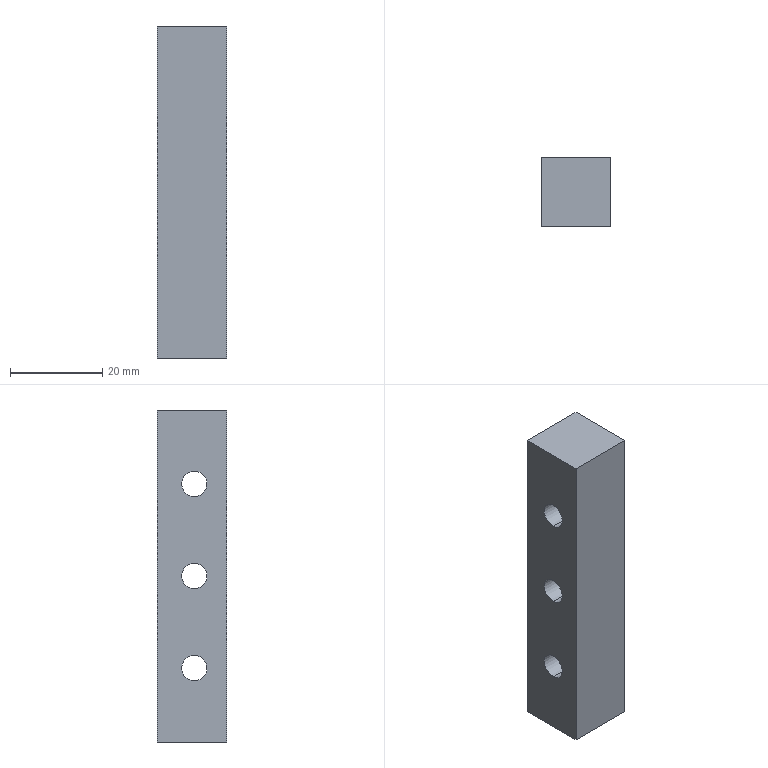Part | SolidWorks | features Extrusion 1, HoleWzd 1 | 1 solid | 21 faces | box 15 x 15 x 72 mm | volume 14194 mm3 | cylinder 12 | plane 9 | commonest cylinder face diameters 5.5 x6 10 x6
STEP:
#1=CARTESIAN_POINT('',(9.3,-0.5,25.));
#2=VERTEX_POINT('',#1);
#3=CARTESIAN_POINT('',(9.3,-0.5,15.));
#4=VERTEX_POINT('',#3);
#5=CARTESIAN_POINT('',(9.3,-0.5,20.));
#6=DIRECTION('',(1.,0.,0.));
#7=DIRECTION('',(0.,0.,-1.));
#8=AXIS2_PLACEMENT_3D('',#5,#6,#7);
#9=CIRCLE('',#8,5.);
#10=EDGE_CURVE('',#2,#4,#9,.T.);
#11=ORIENTED_EDGE('',*,*,#10,.F.);
#12=CARTESIAN_POINT('',(15.,-0.5,25.));
#13=VERTEX_POINT('',#12);
#14=CARTESIAN_POINT('',(15.,-0.5,25.));
#15=DIRECTION('',(1.,0.,0.));
#16=VECTOR('',#15,1000.);
#17=LINE('',#14,#16);
#18=EDGE_CURVE('',#2,#13,#17,.T.);
#19=ORIENTED_EDGE('',*,*,#18,.T.);
#20=CARTESIAN_POINT('',(15.,-0.5,15.));
#21=VERTEX_POINT('',#20);
#22=CARTESIAN_POINT('',(15.,-0.5,20.));
#23=DIRECTION('',(1.,0.,0.));
#24=DIRECTION('',(0.,0.,-1.));
#25=AXIS2_PLACEMENT_3D('',#22,#23,#24);
#26=CIRCLE('',#25,5.);
#27=EDGE_CURVE('',#13,#21,#26,.T.);
#28=ORIENTED_EDGE('',*,*,#27,.T.);
#29=CARTESIAN_POINT('',(15.,-0.5,15.));
#30=DIRECTION('',(1.,0.,0.));
#31=VECTOR('',#30,1000.);
#32=LINE('',#29,#31);
#33=EDGE_CURVE('',#4,#21,#32,.T.);
#34=ORIENTED_EDGE('',*,*,#33,.F.);
#35=EDGE_LOOP('',(#11,#19,#28,#34));
#36=FACE_OUTER_BOUND('',#35,.T.);
#37=CARTESIAN_POINT('',(15.,-0.5,20.));
#38=DIRECTION('',(1.,0.,0.));
#39=DIRECTION('',(0.,0.,-1.));
#40=AXIS2_PLACEMENT_3D('',#37,#38,#39);
#41=CYLINDRICAL_SURFACE('',#40,5.);
#42=ADVANCED_FACE('',(#36),#41,.F.);
#43=CARTESIAN_POINT('',(0.,-0.5,22.75));
#44=VERTEX_POINT('',#43);
#45=CARTESIAN_POINT('',(0.,-0.5,17.25));
#46=VERTEX_POINT('',#45);
#47=CARTESIAN_POINT('',(0.,-0.5,20.));
#48=DIRECTION('',(1.,0.,0.));
#49=DIRECTION('',(0.,0.,-1.));
#50=AXIS2_PLACEMENT_3D('',#47,#48,#49);
#51=CIRCLE('',#50,2.75);
#52=EDGE_CURVE('',#44,#46,#51,.T.);
#53=ORIENTED_EDGE('',*,*,#52,.F.);
#54=CARTESIAN_POINT('',(9.3,-0.5,22.75));
#55=VERTEX_POINT('',#54);
#56=CARTESIAN_POINT('',(15.,-0.5,22.75));
#57=DIRECTION('',(1.,0.,0.));
#58=VECTOR('',#57,1000.);
#59=LINE('',#56,#58);
#60=EDGE_CURVE('',#44,#55,#59,.T.);
#61=ORIENTED_EDGE('',*,*,#60,.T.);
#62=CARTESIAN_POINT('',(9.3,-0.5,17.25));
#63=VERTEX_POINT('',#62);
#64=CARTESIAN_POINT('',(9.3,-0.5,20.));
#65=DIRECTION('',(1.,0.,0.));
#66=DIRECTION('',(0.,0.,-1.));
#67=AXIS2_PLACEMENT_3D('',#64,#65,#66);
#68=CIRCLE('',#67,2.75);
#69=EDGE_CURVE('',#55,#63,#68,.T.);
#70=ORIENTED_EDGE('',*,*,#69,.T.);
#71=CARTESIAN_POINT('',(15.,-0.5,17.25));
#72=DIRECTION('',(1.,0.,0.));
#73=VECTOR('',#72,1000.);
#74=LINE('',#71,#73);
#75=EDGE_CURVE('',#46,#63,#74,.T.);
#76=ORIENTED_EDGE('',*,*,#75,.F.);
#77=EDGE_LOOP('',(#53,#61,#70,#76));
#78=FACE_OUTER_BOUND('',#77,.T.);
#79=CARTESIAN_POINT('',(15.,-0.5,20.));
#80=DIRECTION('',(1.,0.,0.));
#81=DIRECTION('',(0.,0.,-1.));
#82=AXIS2_PLACEMENT_3D('',#79,#80,#81);
#83=CYLINDRICAL_SURFACE('',#82,2.75);
#84=ADVANCED_FACE('',(#78),#83,.F.);
#85=CARTESIAN_POINT('',(9.3,-0.5,5.));
#86=VERTEX_POINT('',#85);
#87=CARTESIAN_POINT('',(9.3,-0.5,-5.));
#88=VERTEX_POINT('',#87);
#89=CARTESIAN_POINT('',(9.3,-0.5,0.));
#90=DIRECTION('',(1.,0.,0.));
#91=DIRECTION('',(0.,0.,-1.));
#92=AXIS2_PLACEMENT_3D('',#89,#90,#91);
#93=CIRCLE('',#92,5.);
#94=EDGE_CURVE('',#86,#88,#93,.T.);
#95=ORIENTED_EDGE('',*,*,#94,.F.);
#96=CARTESIAN_POINT('',(15.,-0.5,5.));
#97=VERTEX_POINT('',#96);
#98=CARTESIAN_POINT('',(15.,-0.5,5.));
#99=DIRECTION('',(1.,0.,0.));
#100=VECTOR('',#99,1000.);
#101=LINE('',#98,#100);
#102=EDGE_CURVE('',#86,#97,#101,.T.);
#103=ORIENTED_EDGE('',*,*,#102,.T.);
#104=CARTESIAN_POINT('',(15.,-0.5,-5.));
#105=VERTEX_POINT('',#104);
#106=CARTESIAN_POINT('',(15.,-0.5,0.));
#107=DIRECTION('',(1.,0.,0.));
#108=DIRECTION('',(0.,0.,-1.));
#109=AXIS2_PLACEMENT_3D('',#106,#107,#108);
#110=CIRCLE('',#109,5.);
#111=EDGE_CURVE('',#97,#105,#110,.T.);
#112=ORIENTED_EDGE('',*,*,#111,.T.);
#113=CARTESIAN_POINT('',(15.,-0.5,-5.));
#114=DIRECTION('',(1.,0.,0.));
#115=VECTOR('',#114,1000.);
#116=LINE('',#113,#115);
#117=EDGE_CURVE('',#88,#105,#116,.T.);
#118=ORIENTED_EDGE('',*,*,#117,.F.);
#119=EDGE_LOOP('',(#95,#103,#112,#118));
#120=FACE_OUTER_BOUND('',#119,.T.);
#121=CARTESIAN_POINT('',(15.,-0.5,0.));
#122=DIRECTION('',(1.,0.,0.));
#123=DIRECTION('',(0.,0.,-1.));
#124=AXIS2_PLACEMENT_3D('',#121,#122,#123);
#125=CYLINDRICAL_SURFACE('',#124,5.);
#126=ADVANCED_FACE('',(#120),#125,.F.);
#127=CARTESIAN_POINT('',(0.,-0.5,2.75));
#128=VERTEX_POINT('',#127);
#129=CARTESIAN_POINT('',(0.,-0.5,-2.75));
#130=VERTEX_POINT('',#129);
#131=CARTESIAN_POINT('',(0.,-0.5,0.));
#132=DIRECTION('',(1.,0.,0.));
#133=DIRECTION('',(0.,0.,-1.));
#134=AXIS2_PLACEMENT_3D('',#131,#132,#133);
#135=CIRCLE('',#134,2.75);
#136=EDGE_CURVE('',#128,#130,#135,.T.);
#137=ORIENTED_EDGE('',*,*,#136,.F.);
#138=CARTESIAN_POINT('',(9.3,-0.5,2.75));
#139=VERTEX_POINT('',#138);
#140=CARTESIAN_POINT('',(15.,-0.5,2.75));
#141=DIRECTION('',(1.,0.,0.));
#142=VECTOR('',#141,1000.);
#143=LINE('',#140,#142);
#144=EDGE_CURVE('',#128,#139,#143,.T.);
#145=ORIENTED_EDGE('',*,*,#144,.T.);
#146=CARTESIAN_POINT('',(9.3,-0.5,-2.75));
#147=VERTEX_POINT('',#146);
#148=CARTESIAN_POINT('',(9.3,-0.5,0.));
#149=DIRECTION('',(1.,0.,0.));
#150=DIRECTION('',(0.,0.,-1.));
#151=AXIS2_PLACEMENT_3D('',#148,#149,#150);
#152=CIRCLE('',#151,2.75);
#153=EDGE_CURVE('',#139,#147,#152,.T.);
#154=ORIENTED_EDGE('',*,*,#153,.T.);
#155=CARTESIAN_POINT('',(15.,-0.5,-2.75));
#156=DIRECTION('',(1.,0.,0.));
#157=VECTOR('',#156,1000.);
#158=LINE('',#155,#157);
#159=EDGE_CURVE('',#130,#147,#158,.T.);
#160=ORIENTED_EDGE('',*,*,#159,.F.);
#161=EDGE_LOOP('',(#137,#145,#154,#160));
#162=FACE_OUTER_BOUND('',#161,.T.);
#163=CARTESIAN_POINT('',(15.,-0.5,0.));
#164=DIRECTION('',(1.,0.,0.));
#165=DIRECTION('',(0.,0.,-1.));
#166=AXIS2_PLACEMENT_3D('',#163,#164,#165);
#167=CYLINDRICAL_SURFACE('',#166,2.75);
#168=ADVANCED_FACE('',(#162),#167,.F.);
#169=CARTESIAN_POINT('',(9.3,-0.5,-15.));
#170=VERTEX_POINT('',#169);
#171=CARTESIAN_POINT('',(9.3,-0.5,-25.));
#172=VERTEX_POINT('',#171);
#173=CARTESIAN_POINT('',(9.3,-0.5,-20.));
#174=DIRECTION('',(1.,0.,0.));
#175=DIRECTION('',(0.,0.,-1.));
#176=AXIS2_PLACEMENT_3D('',#173,#174,#175);
#177=CIRCLE('',#176,5.);
#178=EDGE_CURVE('',#170,#172,#177,.T.);
#179=ORIENTED_EDGE('',*,*,#178,.F.);
#180=CARTESIAN_POINT('',(15.,-0.5,-15.));
#181=VERTEX_POINT('',#180);
#182=CARTESIAN_POINT('',(15.,-0.5,-15.));
#183=DIRECTION('',(1.,0.,0.));
#184=VECTOR('',#183,1000.);
#185=LINE('',#182,#184);
#186=EDGE_CURVE('',#170,#181,#185,.T.);
#187=ORIENTED_EDGE('',*,*,#186,.T.);
#188=CARTESIAN_POINT('',(15.,-0.5,-25.));
#189=VERTEX_POINT('',#188);
#190=CARTESIAN_POINT('',(15.,-0.5,-20.));
#191=DIRECTION('',(1.,0.,0.));
#192=DIRECTION('',(0.,0.,-1.));
#193=AXIS2_PLACEMENT_3D('',#190,#191,#192);
#194=CIRCLE('',#193,5.);
#195=EDGE_CURVE('',#181,#189,#194,.T.);
#196=ORIENTED_EDGE('',*,*,#195,.T.);
#197=CARTESIAN_POINT('',(15.,-0.5,-25.));
#198=DIRECTION('',(1.,0.,0.));
#199=VECTOR('',#198,1000.);
#200=LINE('',#197,#199);
#201=EDGE_CURVE('',#172,#189,#200,.T.);
#202=ORIENTED_EDGE('',*,*,#201,.F.);
#203=EDGE_LOOP('',(#179,#187,#196,#202));
#204=FACE_OUTER_BOUND('',#203,.T.);
#205=CARTESIAN_POINT('',(15.,-0.5,-20.));
#206=DIRECTION('',(1.,0.,0.));
#207=DIRECTION('',(0.,0.,-1.));
#208=AXIS2_PLACEMENT_3D('',#205,#206,#207);
#209=CYLINDRICAL_SURFACE('',#208,5.);
#210=ADVANCED_FACE('',(#204),#209,.F.);
#211=CARTESIAN_POINT('',(0.,-0.5,-17.25));
#212=VERTEX_POINT('',#211);
#213=CARTESIAN_POINT('',(0.,-0.5,-22.75));
#214=VERTEX_POINT('',#213);
#215=CARTESIAN_POINT('',(0.,-0.5,-20.));
#216=DIRECTION('',(1.,0.,0.));
#217=DIRECTION('',(0.,0.,-1.));
#218=AXIS2_PLACEMENT_3D('',#215,#216,#217);
#219=CIRCLE('',#218,2.75);
#220=EDGE_CURVE('',#212,#214,#219,.T.);
#221=ORIENTED_EDGE('',*,*,#220,.F.);
#222=CARTESIAN_POINT('',(9.3,-0.5,-17.25));
#223=VERTEX_POINT('',#222);
#224=CARTESIAN_POINT('',(15.,-0.5,-17.25));
#225=DIRECTION('',(1.,0.,0.));
#226=VECTOR('',#225,1000.);
#227=LINE('',#224,#226);
#228=EDGE_CURVE('',#212,#223,#227,.T.);
#229=ORIENTED_EDGE('',*,*,#228,.T.);
#230=CARTESIAN_POINT('',(9.3,-0.5,-22.75));
#231=VERTEX_POINT('',#230);
#232=CARTESIAN_POINT('',(9.3,-0.5,-20.));
#233=DIRECTION('',(1.,0.,0.));
#234=DIRECTION('',(0.,0.,-1.));
#235=AXIS2_PLACEMENT_3D('',#232,#233,#234);
#236=CIRCLE('',#235,2.75);
#237=EDGE_CURVE('',#223,#231,#236,.T.);
#238=ORIENTED_EDGE('',*,*,#237,.T.);
#239=CARTESIAN_POINT('',(15.,-0.5,-22.75));
#240=DIRECTION('',(1.,0.,0.));
#241=VECTOR('',#240,1000.);
#242=LINE('',#239,#241);
#243=EDGE_CURVE('',#214,#231,#242,.T.);
#244=ORIENTED_EDGE('',*,*,#243,.F.);
#245=EDGE_LOOP('',(#221,#229,#238,#244));
#246=FACE_OUTER_BOUND('',#245,.T.);
#247=CARTESIAN_POINT('',(15.,-0.5,-20.));
#248=DIRECTION('',(1.,0.,0.));
#249=DIRECTION('',(0.,0.,-1.));
#250=AXIS2_PLACEMENT_3D('',#247,#248,#249);
#251=CYLINDRICAL_SURFACE('',#250,2.75);
#252=ADVANCED_FACE('',(#246),#251,.F.);
#253=CARTESIAN_POINT('',(0.,-7.5,-36.));
#254=VERTEX_POINT('',#253);
#255=CARTESIAN_POINT('',(0.,7.5,-36.));
#256=VERTEX_POINT('',#255);
#257=CARTESIAN_POINT('',(0.,7.5,-36.));
#258=DIRECTION('',(0.,1.,0.));
#259=VECTOR('',#258,1000.);
#260=LINE('',#257,#259);
#261=EDGE_CURVE('',#254,#256,#260,.T.);
#262=ORIENTED_EDGE('',*,*,#261,.T.);
#263=CARTESIAN_POINT('',(15.,7.5,-36.));
#264=VERTEX_POINT('',#263);
#265=CARTESIAN_POINT('',(15.,7.5,-36.));
#266=DIRECTION('',(-1.,0.,0.));
#267=VECTOR('',#266,1000.);
#268=LINE('',#265,#267);
#269=EDGE_CURVE('',#264,#256,#268,.T.);
#270=ORIENTED_EDGE('',*,*,#269,.F.);
#271=CARTESIAN_POINT('',(15.,-7.5,-36.));
#272=VERTEX_POINT('',#271);
#273=CARTESIAN_POINT('',(15.,7.5,-36.));
#274=DIRECTION('',(0.,1.,0.));
#275=VECTOR('',#274,1000.);
#276=LINE('',#273,#275);
#277=EDGE_CURVE('',#272,#264,#276,.T.);
#278=ORIENTED_EDGE('',*,*,#277,.F.);
#279=CARTESIAN_POINT('',(15.,-7.5,-36.));
#280=DIRECTION('',(-1.,0.,0.));
#281=VECTOR('',#280,1000.);
#282=LINE('',#279,#281);
#283=EDGE_CURVE('',#272,#254,#282,.T.);
#284=ORIENTED_EDGE('',*,*,#283,.T.);
#285=EDGE_LOOP('',(#262,#270,#278,#284));
#286=FACE_OUTER_BOUND('',#285,.T.);
#287=CARTESIAN_POINT('',(15.,7.5,-36.));
#288=DIRECTION('',(0.,0.,1.));
#289=DIRECTION('',(1.,0.,0.));
#290=AXIS2_PLACEMENT_3D('',#287,#288,#289);
#291=PLANE('',#290);
#292=ADVANCED_FACE('',(#286),#291,.F.);
#293=CARTESIAN_POINT('',(0.,7.5,36.));
#294=VERTEX_POINT('',#293);
#295=CARTESIAN_POINT('',(0.,7.5,36.));
#296=DIRECTION('',(0.,0.,1.));
#297=VECTOR('',#296,1000.);
#298=LINE('',#295,#297);
#299=EDGE_CURVE('',#256,#294,#298,.T.);
#300=ORIENTED_EDGE('',*,*,#299,.T.);
#301=CARTESIAN_POINT('',(15.,7.5,36.));
#302=VERTEX_POINT('',#301);
#303=CARTESIAN_POINT('',(15.,7.5,36.));
#304=DIRECTION('',(-1.,0.,0.));
#305=VECTOR('',#304,1000.);
#306=LINE('',#303,#305);
#307=EDGE_CURVE('',#302,#294,#306,.T.);
#308=ORIENTED_EDGE('',*,*,#307,.F.);
#309=CARTESIAN_POINT('',(15.,7.5,36.));
#310=DIRECTION('',(0.,0.,1.));
#311=VECTOR('',#310,1000.);
#312=LINE('',#309,#311);
#313=EDGE_CURVE('',#264,#302,#312,.T.);
#314=ORIENTED_EDGE('',*,*,#313,.F.);
#315=ORIENTED_EDGE('',*,*,#269,.T.);
#316=EDGE_LOOP('',(#300,#308,#314,#315));
#317=FACE_OUTER_BOUND('',#316,.T.);
#318=CARTESIAN_POINT('',(15.,7.5,36.));
#319=DIRECTION('',(0.,-1.,0.));
#320=DIRECTION('',(0.,0.,-1.));
#321=AXIS2_PLACEMENT_3D('',#318,#319,#320);
#322=PLANE('',#321);
#323=ADVANCED_FACE('',(#317),#322,.F.);
#324=CARTESIAN_POINT('',(0.,-7.5,36.));
#325=VERTEX_POINT('',#324);
#326=CARTESIAN_POINT('',(0.,7.5,36.));
#327=DIRECTION('',(0.,-1.,0.));
#328=VECTOR('',#327,1000.);
#329=LINE('',#326,#328);
#330=EDGE_CURVE('',#294,#325,#329,.T.);
#331=ORIENTED_EDGE('',*,*,#330,.T.);
#332=CARTESIAN_POINT('',(15.,-7.5,36.));
#333=VERTEX_POINT('',#332);
#334=CARTESIAN_POINT('',(15.,-7.5,36.));
#335=DIRECTION('',(-1.,0.,0.));
#336=VECTOR('',#335,1000.);
#337=LINE('',#334,#336);
#338=EDGE_CURVE('',#333,#325,#337,.T.);
#339=ORIENTED_EDGE('',*,*,#338,.F.);
#340=CARTESIAN_POINT('',(15.,7.5,36.));
#341=DIRECTION('',(0.,-1.,0.));
#342=VECTOR('',#341,1000.);
#343=LINE('',#340,#342);
#344=EDGE_CURVE('',#302,#333,#343,.T.);
#345=ORIENTED_EDGE('',*,*,#344,.F.);
#346=ORIENTED_EDGE('',*,*,#307,.T.);
#347=EDGE_LOOP('',(#331,#339,#345,#346));
#348=FACE_OUTER_BOUND('',#347,.T.);
#349=CARTESIAN_POINT('',(15.,7.5,36.));
#350=DIRECTION('',(0.,0.,-1.));
#351=DIRECTION('',(-1.,0.,0.));
#352=AXIS2_PLACEMENT_3D('',#349,#350,#351);
#353=PLANE('',#352);
#354=ADVANCED_FACE('',(#348),#353,.F.);
#355=CARTESIAN_POINT('',(0.,-7.5,36.));
#356=DIRECTION('',(0.,0.,-1.));
#357=VECTOR('',#356,1000.);
#358=LINE('',#355,#357);
#359=EDGE_CURVE('',#325,#254,#358,.T.);
#360=ORIENTED_EDGE('',*,*,#359,.T.);
#361=ORIENTED_EDGE('',*,*,#283,.F.);
#362=CARTESIAN_POINT('',(15.,-7.5,36.));
#363=DIRECTION('',(0.,0.,-1.));
#364=VECTOR('',#363,1000.);
#365=LINE('',#362,#364);
#366=EDGE_CURVE('',#333,#272,#365,.T.);
#367=ORIENTED_EDGE('',*,*,#366,.F.);
#368=ORIENTED_EDGE('',*,*,#338,.T.);
#369=EDGE_LOOP('',(#360,#361,#367,#368));
#370=FACE_OUTER_BOUND('',#369,.T.);
#371=CARTESIAN_POINT('',(15.,-7.5,36.));
#372=DIRECTION('',(0.,1.,0.));
#373=DIRECTION('',(0.,0.,1.));
#374=AXIS2_PLACEMENT_3D('',#371,#372,#373);
#375=PLANE('',#374);
#376=ADVANCED_FACE('',(#370),#375,.F.);
#377=CARTESIAN_POINT('',(15.,-0.5,20.));
#378=DIRECTION('',(1.,0.,0.));
#379=DIRECTION('',(0.,0.,-1.));
#380=AXIS2_PLACEMENT_3D('',#377,#378,#379);
#381=CIRCLE('',#380,5.);
#382=EDGE_CURVE('',#21,#13,#381,.T.);
#383=ORIENTED_EDGE('',*,*,#382,.F.);
#384=ORIENTED_EDGE('',*,*,#27,.F.);
#385=EDGE_LOOP('',(#383,#384));
#386=FACE_BOUND('',#385,.T.);
#387=CARTESIAN_POINT('',(15.,-0.5,0.));
#388=DIRECTION('',(1.,0.,0.));
#389=DIRECTION('',(0.,0.,-1.));
#390=AXIS2_PLACEMENT_3D('',#387,#388,#389);
#391=CIRCLE('',#390,5.);
#392=EDGE_CURVE('',#105,#97,#391,.T.);
#393=ORIENTED_EDGE('',*,*,#392,.F.);
#394=ORIENTED_EDGE('',*,*,#111,.F.);
#395=EDGE_LOOP('',(#393,#394));
#396=FACE_BOUND('',#395,.T.);
#397=CARTESIAN_POINT('',(15.,-0.5,-20.));
#398=DIRECTION('',(1.,0.,0.));
#399=DIRECTION('',(0.,0.,-1.));
#400=AXIS2_PLACEMENT_3D('',#397,#398,#399);
#401=CIRCLE('',#400,5.);
#402=EDGE_CURVE('',#189,#181,#401,.T.);
#403=ORIENTED_EDGE('',*,*,#402,.F.);
#404=ORIENTED_EDGE('',*,*,#195,.F.);
#405=EDGE_LOOP('',(#403,#404));
#406=FACE_BOUND('',#405,.T.);
#407=ORIENTED_EDGE('',*,*,#277,.T.);
#408=ORIENTED_EDGE('',*,*,#313,.T.);
#409=ORIENTED_EDGE('',*,*,#344,.T.);
#410=ORIENTED_EDGE('',*,*,#366,.T.);
#411=EDGE_LOOP('',(#407,#408,#409,#410));
#412=FACE_OUTER_BOUND('',#411,.T.);
#413=CARTESIAN_POINT('',(15.,0.,0.));
#414=DIRECTION('',(1.,0.,0.));
#415=DIRECTION('',(0.,0.,-1.));
#416=AXIS2_PLACEMENT_3D('',#413,#414,#415);
#417=PLANE('',#416);
#418=ADVANCED_FACE('',(#386,#396,#406,#412),#417,.T.);
#419=CARTESIAN_POINT('',(0.,-0.5,20.));
#420=DIRECTION('',(1.,0.,0.));
#421=DIRECTION('',(0.,0.,-1.));
#422=AXIS2_PLACEMENT_3D('',#419,#420,#421);
#423=CIRCLE('',#422,2.75);
#424=EDGE_CURVE('',#46,#44,#423,.T.);
#425=ORIENTED_EDGE('',*,*,#424,.T.);
#426=ORIENTED_EDGE('',*,*,#52,.T.);
#427=EDGE_LOOP('',(#425,#426));
#428=FACE_BOUND('',#427,.T.);
#429=CARTESIAN_POINT('',(0.,-0.5,0.));
#430=DIRECTION('',(1.,0.,0.));
#431=DIRECTION('',(0.,0.,-1.));
#432=AXIS2_PLACEMENT_3D('',#429,#430,#431);
#433=CIRCLE('',#432,2.75);
#434=EDGE_CURVE('',#130,#128,#433,.T.);
#435=ORIENTED_EDGE('',*,*,#434,.T.);
#436=ORIENTED_EDGE('',*,*,#136,.T.);
#437=EDGE_LOOP('',(#435,#436));
#438=FACE_BOUND('',#437,.T.);
#439=CARTESIAN_POINT('',(0.,-0.5,-20.));
#440=DIRECTION('',(1.,0.,0.));
#441=DIRECTION('',(0.,0.,-1.));
#442=AXIS2_PLACEMENT_3D('',#439,#440,#441);
#443=CIRCLE('',#442,2.75);
#444=EDGE_CURVE('',#214,#212,#443,.T.);
#445=ORIENTED_EDGE('',*,*,#444,.T.);
#446=ORIENTED_EDGE('',*,*,#220,.T.);
#447=EDGE_LOOP('',(#445,#446));
#448=FACE_BOUND('',#447,.T.);
#449=ORIENTED_EDGE('',*,*,#261,.F.);
#450=ORIENTED_EDGE('',*,*,#359,.F.);
#451=ORIENTED_EDGE('',*,*,#330,.F.);
#452=ORIENTED_EDGE('',*,*,#299,.F.);
#453=EDGE_LOOP('',(#449,#450,#451,#452));
#454=FACE_OUTER_BOUND('',#453,.T.);
#455=CARTESIAN_POINT('',(0.,0.,0.));
#456=DIRECTION('',(1.,0.,0.));
#457=DIRECTION('',(0.,0.,-1.));
#458=AXIS2_PLACEMENT_3D('',#455,#456,#457);
#459=PLANE('',#458);
#460=ADVANCED_FACE('',(#428,#438,#448,#454),#459,.F.);
#461=ORIENTED_EDGE('',*,*,#228,.F.);
#462=ORIENTED_EDGE('',*,*,#444,.F.);
#463=ORIENTED_EDGE('',*,*,#243,.T.);
#464=CARTESIAN_POINT('',(9.3,-0.5,-20.));
#465=DIRECTION('',(1.,0.,0.));
#466=DIRECTION('',(0.,0.,-1.));
#467=AXIS2_PLACEMENT_3D('',#464,#465,#466);
#468=CIRCLE('',#467,2.75);
#469=EDGE_CURVE('',#231,#223,#468,.T.);
#470=ORIENTED_EDGE('',*,*,#469,.T.);
#471=EDGE_LOOP('',(#461,#462,#463,#470));
#472=FACE_OUTER_BOUND('',#471,.T.);
#473=CARTESIAN_POINT('',(15.,-0.5,-20.));
#474=DIRECTION('',(1.,0.,0.));
#475=DIRECTION('',(0.,0.,-1.));
#476=AXIS2_PLACEMENT_3D('',#473,#474,#475);
#477=CYLINDRICAL_SURFACE('',#476,2.75);
#478=ADVANCED_FACE('',(#472),#477,.F.);
#479=ORIENTED_EDGE('',*,*,#469,.F.);
#480=ORIENTED_EDGE('',*,*,#237,.F.);
#481=EDGE_LOOP('',(#479,#480));
#482=FACE_BOUND('',#481,.T.);
#483=CARTESIAN_POINT('',(9.3,-0.5,-20.));
#484=DIRECTION('',(1.,0.,0.));
#485=DIRECTION('',(0.,0.,-1.));
#486=AXIS2_PLACEMENT_3D('',#483,#484,#485);
#487=CIRCLE('',#486,5.);
#488=EDGE_CURVE('',#172,#170,#487,.T.);
#489=ORIENTED_EDGE('',*,*,#488,.T.);
#490=ORIENTED_EDGE('',*,*,#178,.T.);
#491=EDGE_LOOP('',(#489,#490));
#492=FACE_OUTER_BOUND('',#491,.T.);
#493=CARTESIAN_POINT('',(9.3,2.25,-20.));
#494=DIRECTION('',(-1.,0.,0.));
#495=DIRECTION('',(0.,0.,1.));
#496=AXIS2_PLACEMENT_3D('',#493,#494,#495);
#497=PLANE('',#496);
#498=ADVANCED_FACE('',(#482,#492),#497,.F.);
#499=ORIENTED_EDGE('',*,*,#186,.F.);
#500=ORIENTED_EDGE('',*,*,#488,.F.);
#501=ORIENTED_EDGE('',*,*,#201,.T.);
#502=ORIENTED_EDGE('',*,*,#402,.T.);
#503=EDGE_LOOP('',(#499,#500,#501,#502));
#504=FACE_OUTER_BOUND('',#503,.T.);
#505=CARTESIAN_POINT('',(15.,-0.5,-20.));
#506=DIRECTION('',(1.,0.,0.));
#507=DIRECTION('',(0.,0.,-1.));
#508=AXIS2_PLACEMENT_3D('',#505,#506,#507);
#509=CYLINDRICAL_SURFACE('',#508,5.);
#510=ADVANCED_FACE('',(#504),#509,.F.);
#511=ORIENTED_EDGE('',*,*,#144,.F.);
#512=ORIENTED_EDGE('',*,*,#434,.F.);
#513=ORIENTED_EDGE('',*,*,#159,.T.);
#514=CARTESIAN_POINT('',(9.3,-0.5,0.));
#515=DIRECTION('',(1.,0.,0.));
#516=DIRECTION('',(0.,0.,-1.));
#517=AXIS2_PLACEMENT_3D('',#514,#515,#516);
#518=CIRCLE('',#517,2.75);
#519=EDGE_CURVE('',#147,#139,#518,.T.);
#520=ORIENTED_EDGE('',*,*,#519,.T.);
#521=EDGE_LOOP('',(#511,#512,#513,#520));
#522=FACE_OUTER_BOUND('',#521,.T.);
#523=CARTESIAN_POINT('',(15.,-0.5,0.));
#524=DIRECTION('',(1.,0.,0.));
#525=DIRECTION('',(0.,0.,-1.));
#526=AXIS2_PLACEMENT_3D('',#523,#524,#525);
#527=CYLINDRICAL_SURFACE('',#526,2.75);
#528=ADVANCED_FACE('',(#522),#527,.F.);
#529=ORIENTED_EDGE('',*,*,#519,.F.);
#530=ORIENTED_EDGE('',*,*,#153,.F.);
#531=EDGE_LOOP('',(#529,#530));
#532=FACE_BOUND('',#531,.T.);
#533=CARTESIAN_POINT('',(9.3,-0.5,0.));
#534=DIRECTION('',(1.,0.,0.));
#535=DIRECTION('',(0.,0.,-1.));
#536=AXIS2_PLACEMENT_3D('',#533,#534,#535);
#537=CIRCLE('',#536,5.);
#538=EDGE_CURVE('',#88,#86,#537,.T.);
#539=ORIENTED_EDGE('',*,*,#538,.T.);
#540=ORIENTED_EDGE('',*,*,#94,.T.);
#541=EDGE_LOOP('',(#539,#540));
#542=FACE_OUTER_BOUND('',#541,.T.);
#543=CARTESIAN_POINT('',(9.3,2.25,0.));
#544=DIRECTION('',(-1.,0.,0.));
#545=DIRECTION('',(0.,0.,1.));
#546=AXIS2_PLACEMENT_3D('',#543,#544,#545);
#547=PLANE('',#546);
#548=ADVANCED_FACE('',(#532,#542),#547,.F.);
#549=ORIENTED_EDGE('',*,*,#102,.F.);
#550=ORIENTED_EDGE('',*,*,#538,.F.);
#551=ORIENTED_EDGE('',*,*,#117,.T.);
#552=ORIENTED_EDGE('',*,*,#392,.T.);
#553=EDGE_LOOP('',(#549,#550,#551,#552));
#554=FACE_OUTER_BOUND('',#553,.T.);
#555=CARTESIAN_POINT('',(15.,-0.5,0.));
#556=DIRECTION('',(1.,0.,0.));
#557=DIRECTION('',(0.,0.,-1.));
#558=AXIS2_PLACEMENT_3D('',#555,#556,#557);
#559=CYLINDRICAL_SURFACE('',#558,5.);
#560=ADVANCED_FACE('',(#554),#559,.F.);
#561=ORIENTED_EDGE('',*,*,#60,.F.);
#562=ORIENTED_EDGE('',*,*,#424,.F.);
#563=ORIENTED_EDGE('',*,*,#75,.T.);
#564=CARTESIAN_POINT('',(9.3,-0.5,20.));
#565=DIRECTION('',(1.,0.,0.));
#566=DIRECTION('',(0.,0.,-1.));
#567=AXIS2_PLACEMENT_3D('',#564,#565,#566);
#568=CIRCLE('',#567,2.75);
#569=EDGE_CURVE('',#63,#55,#568,.T.);
#570=ORIENTED_EDGE('',*,*,#569,.T.);
#571=EDGE_LOOP('',(#561,#562,#563,#570));
#572=FACE_OUTER_BOUND('',#571,.T.);
#573=CARTESIAN_POINT('',(15.,-0.5,20.));
#574=DIRECTION('',(1.,0.,0.));
#575=DIRECTION('',(0.,0.,-1.));
#576=AXIS2_PLACEMENT_3D('',#573,#574,#575);
#577=CYLINDRICAL_SURFACE('',#576,2.75);
#578=ADVANCED_FACE('',(#572),#577,.F.);
#579=ORIENTED_EDGE('',*,*,#569,.F.);
#580=ORIENTED_EDGE('',*,*,#69,.F.);
#581=EDGE_LOOP('',(#579,#580));
#582=FACE_BOUND('',#581,.T.);
#583=CARTESIAN_POINT('',(9.3,-0.5,20.));
#584=DIRECTION('',(1.,0.,0.));
#585=DIRECTION('',(0.,0.,-1.));
#586=AXIS2_PLACEMENT_3D('',#583,#584,#585);
#587=CIRCLE('',#586,5.);
#588=EDGE_CURVE('',#4,#2,#587,.T.);
#589=ORIENTED_EDGE('',*,*,#588,.T.);
#590=ORIENTED_EDGE('',*,*,#10,.T.);
#591=EDGE_LOOP('',(#589,#590));
#592=FACE_OUTER_BOUND('',#591,.T.);
#593=CARTESIAN_POINT('',(9.3,2.25,20.));
#594=DIRECTION('',(-1.,0.,0.));
#595=DIRECTION('',(0.,0.,1.));
#596=AXIS2_PLACEMENT_3D('',#593,#594,#595);
#597=PLANE('',#596);
#598=ADVANCED_FACE('',(#582,#592),#597,.F.);
#599=ORIENTED_EDGE('',*,*,#18,.F.);
#600=ORIENTED_EDGE('',*,*,#588,.F.);
#601=ORIENTED_EDGE('',*,*,#33,.T.);
#602=ORIENTED_EDGE('',*,*,#382,.T.);
#603=EDGE_LOOP('',(#599,#600,#601,#602));
#604=FACE_OUTER_BOUND('',#603,.T.);
#605=CARTESIAN_POINT('',(15.,-0.5,20.));
#606=DIRECTION('',(1.,0.,0.));
#607=DIRECTION('',(0.,0.,-1.));
#608=AXIS2_PLACEMENT_3D('',#605,#606,#607);
#609=CYLINDRICAL_SURFACE('',#608,5.);
#610=ADVANCED_FACE('',(#604),#609,.F.);
#611=CLOSED_SHELL('',(#42,#84,#126,#168,#210,#252,#292,#323,#354,#376,#418,#460,#478,#498,#510,#528,#548,#560,#578,#598,#610));
#612=MANIFOLD_SOLID_BREP('',#611);
#613=CARTESIAN_POINT('',(0.,0.,0.));
#614=DIRECTION('',(0.,0.,1.));
#615=DIRECTION('',(1.,0.,0.));
#616=AXIS2_PLACEMENT_3D('',#613,#614,#615);
#617=(LENGTH_UNIT()NAMED_UNIT(*)SI_UNIT(.MILLI.,.METRE.));
#618=UNCERTAINTY_MEASURE_WITH_UNIT(LENGTH_MEASURE(0.00001),#617,'','');
#619=(NAMED_UNIT(*)PLANE_ANGLE_UNIT()SI_UNIT($,.RADIAN.));
#620=(NAMED_UNIT(*)SI_UNIT($,.STERADIAN.)SOLID_ANGLE_UNIT());
#621=(GEOMETRIC_REPRESENTATION_CONTEXT(3)GLOBAL_UNCERTAINTY_ASSIGNED_CONTEXT((#618))GLOBAL_UNIT_ASSIGNED_CONTEXT((#617,#619,#620))REPRESENTATION_CONTEXT('',''));
#622=ADVANCED_BREP_SHAPE_REPRESENTATION('',(#612,#616),#621);